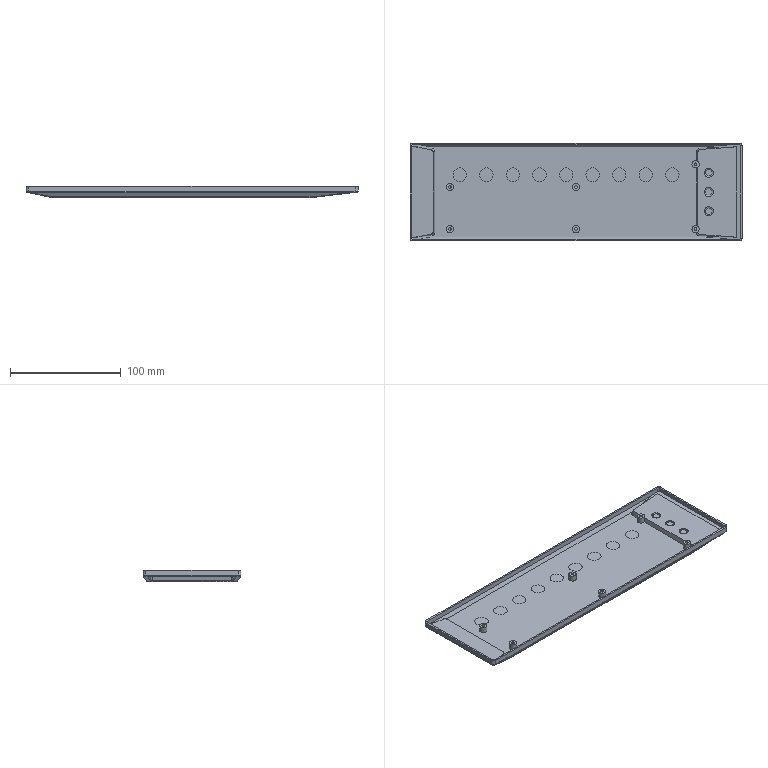Part | 13 solids | 287 faces | box 300 x 88.5 x 10 mm | volume 48360 mm3 | plane 137 | cylinder 118 | spline 12 | cone 12 | sphere 8 | commonest cylinder face diameters 2 x38 12.2 x27 2.5 x12 6.5 x12 6.2 x9 12 x8